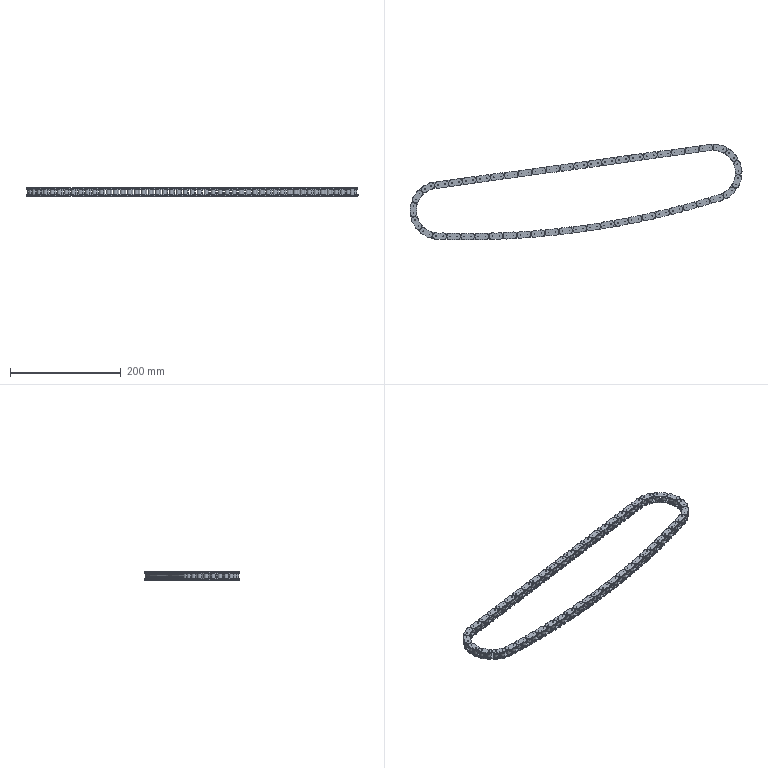Part | SolidWorks | features Boss 3, CurvePattern 2, Chamfer 1, CompositeCurve 1, Extrusion 1, MirrorPattern 1, MirrorSolid 1 | 153 solids | 3060 faces | volume 127327 mm3 | cylinder 2040 | plane 612 | cone 408 | commonest cylinder face diameters 1.035 x816 12.07 x612 55.348 x408 7.92 x204